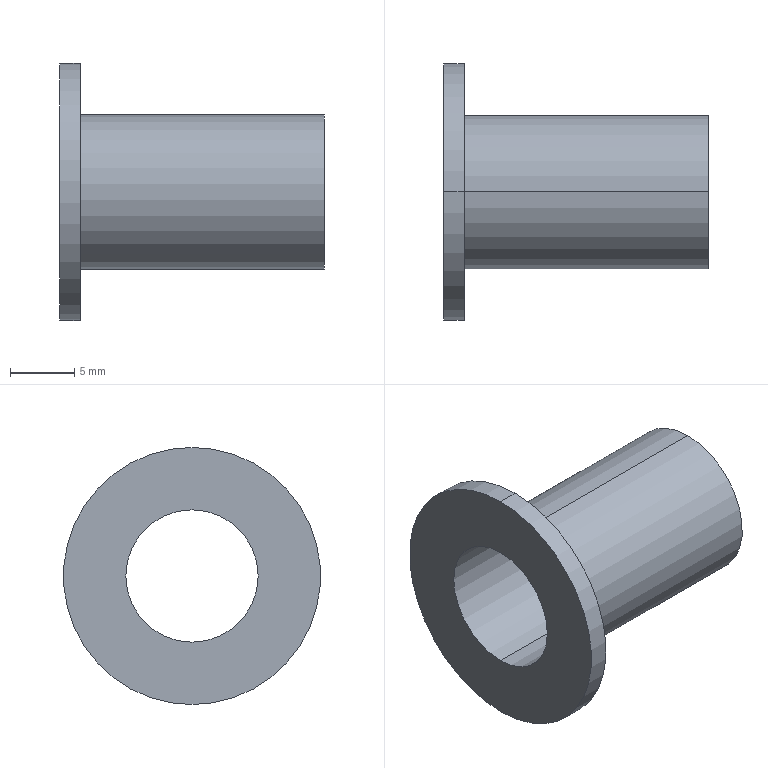Part | SolidWorks | features Revolution 1 | 1 solid | 9 faces | box 20.6 x 20 x 20 mm | volume 935.053 mm3 | cylinder 6 | plane 3 | commonest cylinder face diameters 10.3 x2 12 x2 20 x2
STEP:
#1=CARTESIAN_POINT('',(20.6,0.,6.));
#2=VERTEX_POINT('',#1);
#3=CARTESIAN_POINT('',(20.6,0.,-6.));
#4=VERTEX_POINT('',#3);
#5=CARTESIAN_POINT('',(20.6,0.,0.));
#6=DIRECTION('',(-1.,0.,0.));
#7=DIRECTION('',(0.,0.,1.));
#8=AXIS2_PLACEMENT_3D('',#5,#6,#7);
#9=CIRCLE('',#8,6.);
#10=EDGE_CURVE('',#2,#4,#9,.T.);
#11=ORIENTED_EDGE('',*,*,#10,.T.);
#12=CARTESIAN_POINT('',(1.6,0.,-6.));
#13=VERTEX_POINT('',#12);
#14=CARTESIAN_POINT('',(0.,0.,-6.));
#15=DIRECTION('',(-1.,0.,0.));
#16=VECTOR('',#15,1000.);
#17=LINE('',#14,#16);
#18=EDGE_CURVE('',#4,#13,#17,.T.);
#19=ORIENTED_EDGE('',*,*,#18,.T.);
#20=CARTESIAN_POINT('',(1.6,0.,6.));
#21=VERTEX_POINT('',#20);
#22=CARTESIAN_POINT('',(1.6,0.,0.));
#23=DIRECTION('',(-1.,0.,0.));
#24=DIRECTION('',(0.,0.,1.));
#25=AXIS2_PLACEMENT_3D('',#22,#23,#24);
#26=CIRCLE('',#25,6.);
#27=EDGE_CURVE('',#21,#13,#26,.T.);
#28=ORIENTED_EDGE('',*,*,#27,.F.);
#29=CARTESIAN_POINT('',(0.,0.,6.));
#30=DIRECTION('',(-1.,0.,0.));
#31=VECTOR('',#30,1000.);
#32=LINE('',#29,#31);
#33=EDGE_CURVE('',#2,#21,#32,.T.);
#34=ORIENTED_EDGE('',*,*,#33,.F.);
#35=EDGE_LOOP('',(#11,#19,#28,#34));
#36=FACE_OUTER_BOUND('',#35,.T.);
#37=CARTESIAN_POINT('',(0.,0.,0.));
#38=DIRECTION('',(-1.,0.,0.));
#39=DIRECTION('',(0.,0.,1.));
#40=AXIS2_PLACEMENT_3D('',#37,#38,#39);
#41=CYLINDRICAL_SURFACE('',#40,6.);
#42=ADVANCED_FACE('',(#36),#41,.T.);
#43=CARTESIAN_POINT('',(20.6,0.,-5.15));
#44=VERTEX_POINT('',#43);
#45=CARTESIAN_POINT('',(20.6,0.,5.15));
#46=VERTEX_POINT('',#45);
#47=CARTESIAN_POINT('',(20.6,0.,0.));
#48=DIRECTION('',(-1.,0.,0.));
#49=DIRECTION('',(0.,0.,1.));
#50=AXIS2_PLACEMENT_3D('',#47,#48,#49);
#51=CIRCLE('',#50,5.15);
#52=EDGE_CURVE('',#44,#46,#51,.T.);
#53=ORIENTED_EDGE('',*,*,#52,.F.);
#54=CARTESIAN_POINT('',(0.,0.,-5.15));
#55=VERTEX_POINT('',#54);
#56=CARTESIAN_POINT('',(0.,0.,-5.15));
#57=DIRECTION('',(-1.,0.,0.));
#58=VECTOR('',#57,1000.);
#59=LINE('',#56,#58);
#60=EDGE_CURVE('',#44,#55,#59,.T.);
#61=ORIENTED_EDGE('',*,*,#60,.T.);
#62=CARTESIAN_POINT('',(0.,0.,5.15));
#63=VERTEX_POINT('',#62);
#64=CARTESIAN_POINT('',(0.,0.,0.));
#65=DIRECTION('',(-1.,0.,0.));
#66=DIRECTION('',(0.,0.,1.));
#67=AXIS2_PLACEMENT_3D('',#64,#65,#66);
#68=CIRCLE('',#67,5.15);
#69=EDGE_CURVE('',#55,#63,#68,.T.);
#70=ORIENTED_EDGE('',*,*,#69,.T.);
#71=CARTESIAN_POINT('',(0.,0.,5.15));
#72=DIRECTION('',(-1.,0.,0.));
#73=VECTOR('',#72,1000.);
#74=LINE('',#71,#73);
#75=EDGE_CURVE('',#46,#63,#74,.T.);
#76=ORIENTED_EDGE('',*,*,#75,.F.);
#77=EDGE_LOOP('',(#53,#61,#70,#76));
#78=FACE_OUTER_BOUND('',#77,.T.);
#79=CARTESIAN_POINT('',(0.,0.,0.));
#80=DIRECTION('',(-1.,0.,0.));
#81=DIRECTION('',(0.,0.,1.));
#82=AXIS2_PLACEMENT_3D('',#79,#80,#81);
#83=CYLINDRICAL_SURFACE('',#82,5.15);
#84=ADVANCED_FACE('',(#78),#83,.F.);
#85=CARTESIAN_POINT('',(1.6,0.,10.));
#86=VERTEX_POINT('',#85);
#87=CARTESIAN_POINT('',(1.6,0.,-10.));
#88=VERTEX_POINT('',#87);
#89=CARTESIAN_POINT('',(1.6,0.,0.));
#90=DIRECTION('',(-1.,0.,0.));
#91=DIRECTION('',(0.,0.,1.));
#92=AXIS2_PLACEMENT_3D('',#89,#90,#91);
#93=CIRCLE('',#92,10.);
#94=EDGE_CURVE('',#86,#88,#93,.T.);
#95=ORIENTED_EDGE('',*,*,#94,.T.);
#96=CARTESIAN_POINT('',(0.,0.,-10.));
#97=VERTEX_POINT('',#96);
#98=CARTESIAN_POINT('',(0.,0.,-10.));
#99=DIRECTION('',(-1.,0.,0.));
#100=VECTOR('',#99,1000.);
#101=LINE('',#98,#100);
#102=EDGE_CURVE('',#88,#97,#101,.T.);
#103=ORIENTED_EDGE('',*,*,#102,.T.);
#104=CARTESIAN_POINT('',(0.,0.,10.));
#105=VERTEX_POINT('',#104);
#106=CARTESIAN_POINT('',(0.,0.,0.));
#107=DIRECTION('',(-1.,0.,0.));
#108=DIRECTION('',(0.,0.,1.));
#109=AXIS2_PLACEMENT_3D('',#106,#107,#108);
#110=CIRCLE('',#109,10.);
#111=EDGE_CURVE('',#105,#97,#110,.T.);
#112=ORIENTED_EDGE('',*,*,#111,.F.);
#113=CARTESIAN_POINT('',(0.,0.,10.));
#114=DIRECTION('',(-1.,0.,0.));
#115=VECTOR('',#114,1000.);
#116=LINE('',#113,#115);
#117=EDGE_CURVE('',#86,#105,#116,.T.);
#118=ORIENTED_EDGE('',*,*,#117,.F.);
#119=EDGE_LOOP('',(#95,#103,#112,#118));
#120=FACE_OUTER_BOUND('',#119,.T.);
#121=CARTESIAN_POINT('',(0.,0.,0.));
#122=DIRECTION('',(-1.,0.,0.));
#123=DIRECTION('',(0.,0.,1.));
#124=AXIS2_PLACEMENT_3D('',#121,#122,#123);
#125=CYLINDRICAL_SURFACE('',#124,10.);
#126=ADVANCED_FACE('',(#120),#125,.T.);
#127=ORIENTED_EDGE('',*,*,#94,.F.);
#128=CARTESIAN_POINT('',(1.6,0.,0.));
#129=DIRECTION('',(-1.,0.,0.));
#130=DIRECTION('',(0.,0.,1.));
#131=AXIS2_PLACEMENT_3D('',#128,#129,#130);
#132=CIRCLE('',#131,10.);
#133=EDGE_CURVE('',#88,#86,#132,.T.);
#134=ORIENTED_EDGE('',*,*,#133,.F.);
#135=EDGE_LOOP('',(#127,#134));
#136=FACE_OUTER_BOUND('',#135,.T.);
#137=ORIENTED_EDGE('',*,*,#27,.T.);
#138=CARTESIAN_POINT('',(1.6,0.,0.));
#139=DIRECTION('',(-1.,0.,0.));
#140=DIRECTION('',(0.,0.,1.));
#141=AXIS2_PLACEMENT_3D('',#138,#139,#140);
#142=CIRCLE('',#141,6.);
#143=EDGE_CURVE('',#13,#21,#142,.T.);
#144=ORIENTED_EDGE('',*,*,#143,.T.);
#145=EDGE_LOOP('',(#137,#144));
#146=FACE_BOUND('',#145,.T.);
#147=CARTESIAN_POINT('',(1.6,10.,0.));
#148=DIRECTION('',(-1.,0.,0.));
#149=DIRECTION('',(0.,0.,1.));
#150=AXIS2_PLACEMENT_3D('',#147,#148,#149);
#151=PLANE('',#150);
#152=ADVANCED_FACE('',(#136,#146),#151,.F.);
#153=ORIENTED_EDGE('',*,*,#102,.F.);
#154=ORIENTED_EDGE('',*,*,#133,.T.);
#155=ORIENTED_EDGE('',*,*,#117,.T.);
#156=CARTESIAN_POINT('',(0.,0.,0.));
#157=DIRECTION('',(-1.,0.,0.));
#158=DIRECTION('',(0.,0.,1.));
#159=AXIS2_PLACEMENT_3D('',#156,#157,#158);
#160=CIRCLE('',#159,10.);
#161=EDGE_CURVE('',#97,#105,#160,.T.);
#162=ORIENTED_EDGE('',*,*,#161,.F.);
#163=EDGE_LOOP('',(#153,#154,#155,#162));
#164=FACE_OUTER_BOUND('',#163,.T.);
#165=CARTESIAN_POINT('',(0.,0.,0.));
#166=DIRECTION('',(-1.,0.,0.));
#167=DIRECTION('',(0.,0.,1.));
#168=AXIS2_PLACEMENT_3D('',#165,#166,#167);
#169=CYLINDRICAL_SURFACE('',#168,10.);
#170=ADVANCED_FACE('',(#164),#169,.T.);
#171=CARTESIAN_POINT('',(0.,0.,0.));
#172=DIRECTION('',(-1.,0.,0.));
#173=DIRECTION('',(0.,0.,1.));
#174=AXIS2_PLACEMENT_3D('',#171,#172,#173);
#175=CIRCLE('',#174,5.15);
#176=EDGE_CURVE('',#63,#55,#175,.T.);
#177=ORIENTED_EDGE('',*,*,#176,.F.);
#178=ORIENTED_EDGE('',*,*,#69,.F.);
#179=EDGE_LOOP('',(#177,#178));
#180=FACE_BOUND('',#179,.T.);
#181=ORIENTED_EDGE('',*,*,#111,.T.);
#182=ORIENTED_EDGE('',*,*,#161,.T.);
#183=EDGE_LOOP('',(#181,#182));
#184=FACE_OUTER_BOUND('',#183,.T.);
#185=CARTESIAN_POINT('',(0.,5.15,0.));
#186=DIRECTION('',(1.,0.,0.));
#187=DIRECTION('',(0.,0.,-1.));
#188=AXIS2_PLACEMENT_3D('',#185,#186,#187);
#189=PLANE('',#188);
#190=ADVANCED_FACE('',(#180,#184),#189,.F.);
#191=ORIENTED_EDGE('',*,*,#60,.F.);
#192=CARTESIAN_POINT('',(20.6,0.,0.));
#193=DIRECTION('',(-1.,0.,0.));
#194=DIRECTION('',(0.,0.,1.));
#195=AXIS2_PLACEMENT_3D('',#192,#193,#194);
#196=CIRCLE('',#195,5.15);
#197=EDGE_CURVE('',#46,#44,#196,.T.);
#198=ORIENTED_EDGE('',*,*,#197,.F.);
#199=ORIENTED_EDGE('',*,*,#75,.T.);
#200=ORIENTED_EDGE('',*,*,#176,.T.);
#201=EDGE_LOOP('',(#191,#198,#199,#200));
#202=FACE_OUTER_BOUND('',#201,.T.);
#203=CARTESIAN_POINT('',(0.,0.,0.));
#204=DIRECTION('',(-1.,0.,0.));
#205=DIRECTION('',(0.,0.,1.));
#206=AXIS2_PLACEMENT_3D('',#203,#204,#205);
#207=CYLINDRICAL_SURFACE('',#206,5.15);
#208=ADVANCED_FACE('',(#202),#207,.F.);
#209=ORIENTED_EDGE('',*,*,#10,.F.);
#210=CARTESIAN_POINT('',(20.6,0.,0.));
#211=DIRECTION('',(-1.,0.,0.));
#212=DIRECTION('',(0.,0.,1.));
#213=AXIS2_PLACEMENT_3D('',#210,#211,#212);
#214=CIRCLE('',#213,6.);
#215=EDGE_CURVE('',#4,#2,#214,.T.);
#216=ORIENTED_EDGE('',*,*,#215,.F.);
#217=EDGE_LOOP('',(#209,#216));
#218=FACE_OUTER_BOUND('',#217,.T.);
#219=ORIENTED_EDGE('',*,*,#197,.T.);
#220=ORIENTED_EDGE('',*,*,#52,.T.);
#221=EDGE_LOOP('',(#219,#220));
#222=FACE_BOUND('',#221,.T.);
#223=CARTESIAN_POINT('',(20.6,6.,0.));
#224=DIRECTION('',(-1.,0.,0.));
#225=DIRECTION('',(0.,0.,1.));
#226=AXIS2_PLACEMENT_3D('',#223,#224,#225);
#227=PLANE('',#226);
#228=ADVANCED_FACE('',(#218,#222),#227,.F.);
#229=ORIENTED_EDGE('',*,*,#18,.F.);
#230=ORIENTED_EDGE('',*,*,#215,.T.);
#231=ORIENTED_EDGE('',*,*,#33,.T.);
#232=ORIENTED_EDGE('',*,*,#143,.F.);
#233=EDGE_LOOP('',(#229,#230,#231,#232));
#234=FACE_OUTER_BOUND('',#233,.T.);
#235=CARTESIAN_POINT('',(0.,0.,0.));
#236=DIRECTION('',(-1.,0.,0.));
#237=DIRECTION('',(0.,0.,1.));
#238=AXIS2_PLACEMENT_3D('',#235,#236,#237);
#239=CYLINDRICAL_SURFACE('',#238,6.);
#240=ADVANCED_FACE('',(#234),#239,.T.);
#241=CLOSED_SHELL('',(#42,#84,#126,#152,#170,#190,#208,#228,#240));
#242=MANIFOLD_SOLID_BREP('',#241);
#243=CARTESIAN_POINT('',(0.,0.,0.));
#244=DIRECTION('',(0.,0.,1.));
#245=DIRECTION('',(1.,0.,0.));
#246=AXIS2_PLACEMENT_3D('',#243,#244,#245);
#247=(LENGTH_UNIT()NAMED_UNIT(*)SI_UNIT(.MILLI.,.METRE.));
#248=UNCERTAINTY_MEASURE_WITH_UNIT(LENGTH_MEASURE(0.00001),#247,'','');
#249=(NAMED_UNIT(*)PLANE_ANGLE_UNIT()SI_UNIT($,.RADIAN.));
#250=(NAMED_UNIT(*)SI_UNIT($,.STERADIAN.)SOLID_ANGLE_UNIT());
#251=(GEOMETRIC_REPRESENTATION_CONTEXT(3)GLOBAL_UNCERTAINTY_ASSIGNED_CONTEXT((#248))GLOBAL_UNIT_ASSIGNED_CONTEXT((#247,#249,#250))REPRESENTATION_CONTEXT('',''));
#252=ADVANCED_BREP_SHAPE_REPRESENTATION('',(#242,#246),#251);